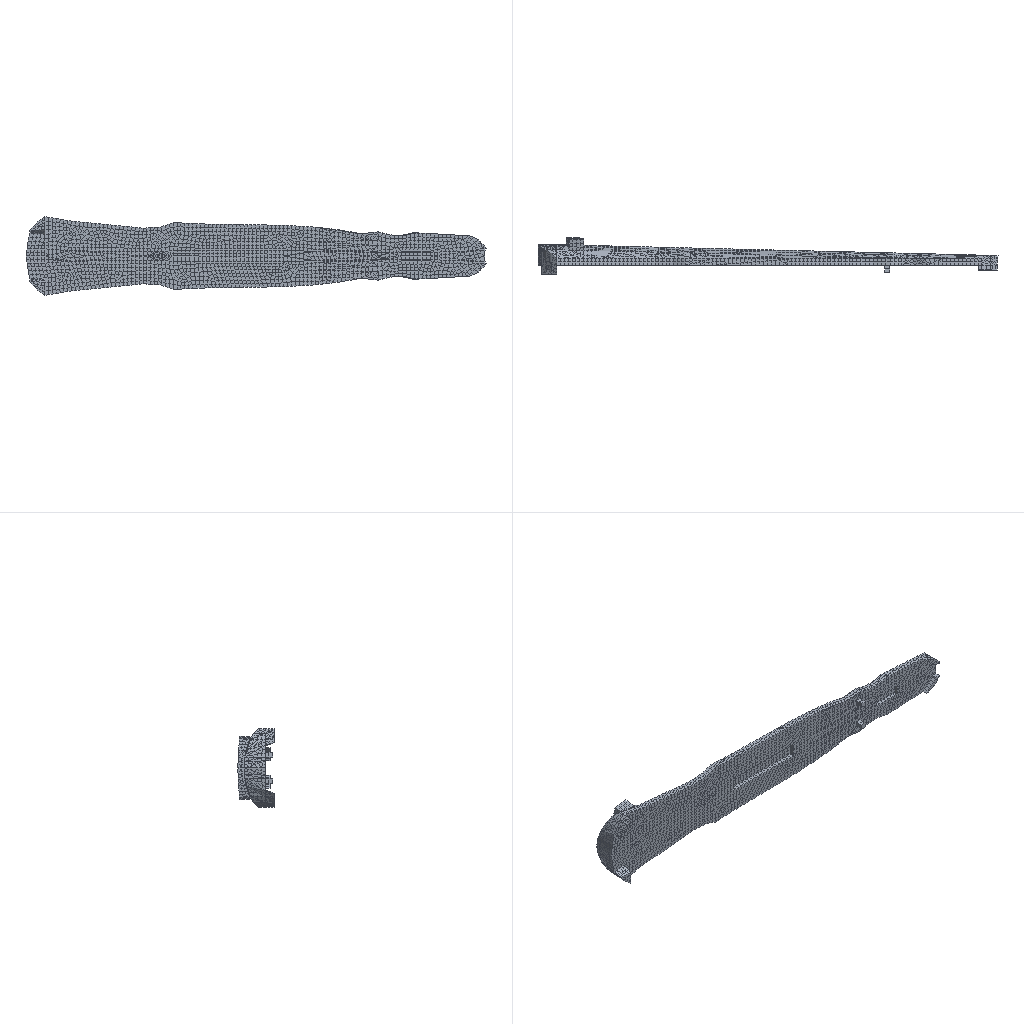Simulation study | abaqus
Set-up summary:
category,name,step,type,value,unit,region
solver,abaqus
solver,version,,,Abaqus/Standard 2020
units,not stated in the deck,,not stated
analysis,deck,,static,modal; static
load_step,Step-1,Step-1,static,nlgeom=True
load_step,Step-2,Step-2,modal,nlgeom=False
contact,interactions,,,general=0 pairs=0 ties=0
load_step,requested,,,2
mesh,nodes,,,6082
mesh,elements,,,6440
element_type,S3,,shell,724
element_type,S4R,,shell,5716
load,load commands in deck,,count,3
bc,support commands in deck,,count,1
material,MATERIAL-1,,in results
check,setup vs results,,match,"per instance, exact: element labels, types and connectivity; labels of the nodes the elements use; coordinates of those nodes at SINGLE_PRECISION in 1 of 1 instance(s)"
Abaqus input file, long lists of numbers shortened:
*Heading
** Job name: Job-2 Model name: Model-1-Copy
** Generated by: Abaqus/CAE 2020
*Preprint, echo=NO, model=NO, history=NO, contact=NO
**
** PARTS
**
*Part, name=work-9
*Node
      1,  -28.42, -0.02369,   7.003
      2,   -46.71, -0.02369,   8.803
** (6080 more lines like these left out)
*Element, type=S4R
 1,    1,  395, 3841,  430
 2,  395,  396, 3842, 3841
** (5714 more lines like these left out)
*Element, type=S3
689,  960,  182,  961
690, 4094,  948,  949
** (722 more lines like these left out)
*Nset, nset=Set-3, generate
    1,  6082,     1
*Elset, elset=Set-3, generate
    1,  6440,     1
** Section: Section-2
*Shell Section, elset=Set-3, material=Material-1
1., 5
*End Part
**
**
** ASSEMBLY
**
*Assembly, name=Assembly
**
*Instance, name=work-9-1, part=work-9
*End Instance
**
*Nset, nset=Set-1, instance=work-9-1
   22,   23,  100,  101,  114,  117,  118,  121,  124,  125,  126,  129,  152,  153,  155,  156
  158,  159,  162,  164,  166,  169,  171,  173,  175,  176,  178,  180,  224,  227,  228,  310
** (4 more lines like these left out)
*Elset, elset=Set-1, instance=work-9-1
  598,  607, 2050, 2051, 2052, 2053, 2054, 2055, 2056, 2057, 2058, 2059, 2060, 2061, 2062, 2063
 2064, 2065, 4922, 4923, 4924, 4925, 4926, 4927, 4928, 4929, 4930, 4931, 4932, 4933, 4934, 4935
** (2 more lines like these left out)
*Nset, nset=Set-2, instance=work-9-1
   22,   23,  100,  101,  114,  117,  118,  121,  124,  125,  126,  129,  152,  153,  155,  156
  158,  159,  162,  164,  166,  169,  171,  173,  175,  176,  178,  180,  224,  227,  228,  310
** (4 more lines like these left out)
*Elset, elset=Set-2, instance=work-9-1
  598,  607, 2050, 2051, 2052, 2053, 2054, 2055, 2056, 2057, 2058, 2059, 2060, 2061, 2062, 2063
 2064, 2065, 4922, 4923, 4924, 4925, 4926, 4927, 4928, 4929, 4930, 4931, 4932, 4933, 4934, 4935
** (2 more lines like these left out)
*Elset, elset=_Surf-1_SPOS, internal, instance=work-9-1
   71,   72,   73,   74,   75,   76,   77,   78,   79,   80,   81,   82,  317,  318,  319,  320
  321,  322,  323,  324,  325,  326,  327,  328, 1612, 1613, 1614, 1615, 1697, 1698, 1699, 1841
** (2 more lines like these left out)
*Surface, type=ELEMENT, name=Surf-1
_Surf-1_SPOS, SPOS
*Elset, elset=_Surf-2_SPOS, internal, instance=work-9-1
 594, 595, 603, 604
*Surface, type=ELEMENT, name=Surf-2
_Surf-2_SPOS, SPOS
*Elset, elset=_Surf-3_SPOS, internal, instance=work-9-1
 6096, 6097, 6121, 6122, 6137, 6138, 6139, 6140, 6165, 6166, 6167, 6168, 6169, 6184, 6185, 6186
 6187, 6188, 6203, 6204, 6205, 6206, 6221, 6222, 6237, 6238
*Surface, type=ELEMENT, name=Surf-3
_Surf-3_SPOS, SPOS
*End Assembly
**
** MATERIALS
**
*Material, name=Material-1
*Density
 1.8e-09,
*Elastic
15000., 0.25
** ----------------------------------------------------------------
**
** STEP: Step-1
**
*Step, name=Step-1, nlgeom=YES
*Static
0.01, 1., 1e-05, 0.1
**
** BOUNDARY CONDITIONS
**
** Name: BC-1 Type: 对称/反对称/完全固定
*Boundary
Set-2, ENCASTRE
**
** LOADS
**
** Name: Load-1   Type: Pressure
*Dsload
Surf-1, P, 0.01
** Name: Load-2   Type: Pressure
*Dsload
Surf-2, P, 0.01
** Name: Load-3   Type: Pressure
*Dsload
Surf-3, P, 0.001
**
** OUTPUT REQUESTS
**
*Restart, write, frequency=0
**
** FIELD OUTPUT: F-Output-1
**
*Output, field
*Node Output
CF, RF, U, V
*Element Output, directions=YES
E, LE, MISES, MISESMAX, MISESONLY, NE, PE, PEEQ, PEMAG, PRESSONLY, S, SEQUT, YIELDPOT
*Contact Output
CDISP, CSTRESS
**
** HISTORY OUTPUT: H-Output-1
**
*Output, history, variable=PRESELECT
*End Step
** ----------------------------------------------------------------
**
** STEP: Step-2
**
*Step, name=Step-2, nlgeom=NO, perturbation
*Frequency, eigensolver=Lanczos, sim, acoustic coupling=on, normalization=mass
10, , , , ,
**
** OUTPUT REQUESTS
**
*Restart, write, frequency=0
**
** FIELD OUTPUT: F-Output-2
**
*Output, field, variable=PRESELECT
*End Step
Results summary:
result,step,,completed,increments=15 time=1.0/1.0
result,step,,partial,increments=0 time=0.0/1e-36
result,analysis,,,modal
result,last_loadstep,,,2
result,analysis steps,,count,2
result,primary field,,,"U, UR"